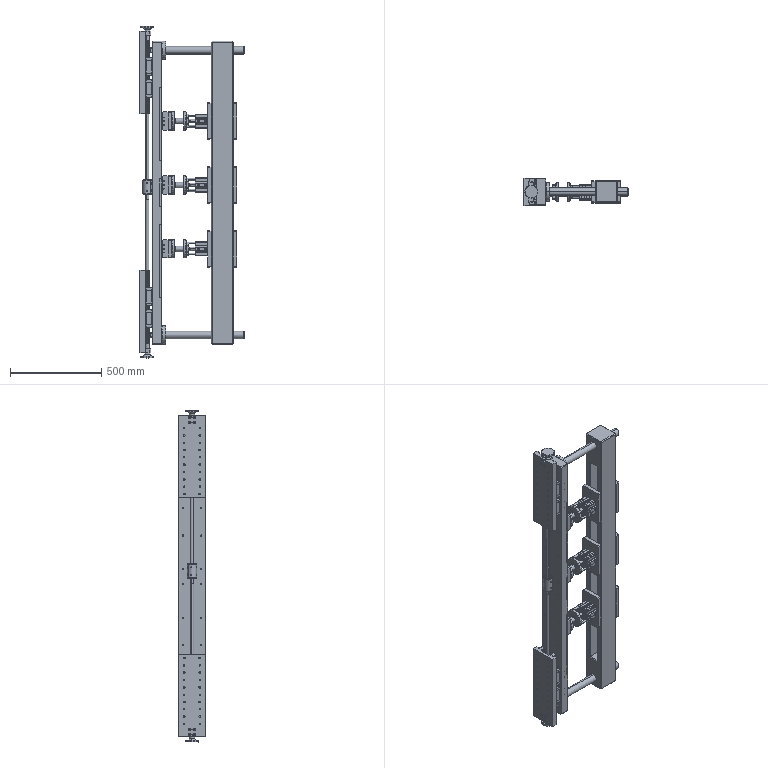Part | SolidWorks | features ReferencePattern 12, CompositeCurve 4, LocalLPattern 1 | 57 solids | 5716 faces | volume 40703347 mm3 | plane 3403 | cylinder 1551 | spline 504 | cone 242 | torus 16 | commonest cylinder face diameters 9 x226 15 x194 1.2 x144 6.8 x138 0.4 x123 8 x64